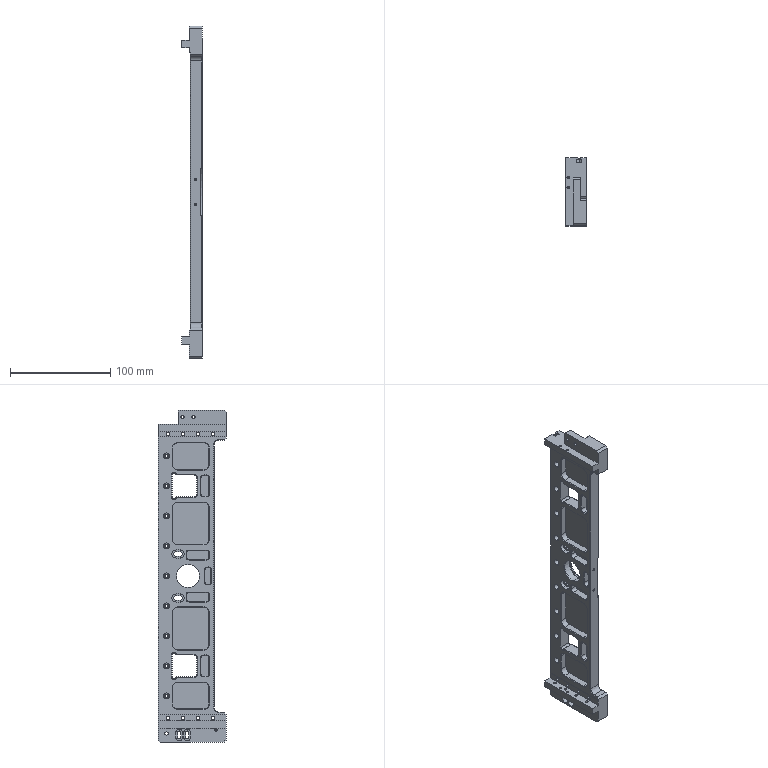Part | NX | features BREP 1 | 1 solid | 470 faces | box 20.5 x 68 x 332 mm | volume 153235 mm3 | plane 205 | cylinder 175 | cone 50 | spline 40 | commonest cylinder face diameters 3.4 x40 2.5 x26 6 x22 7 x22 10 x20 4 x9